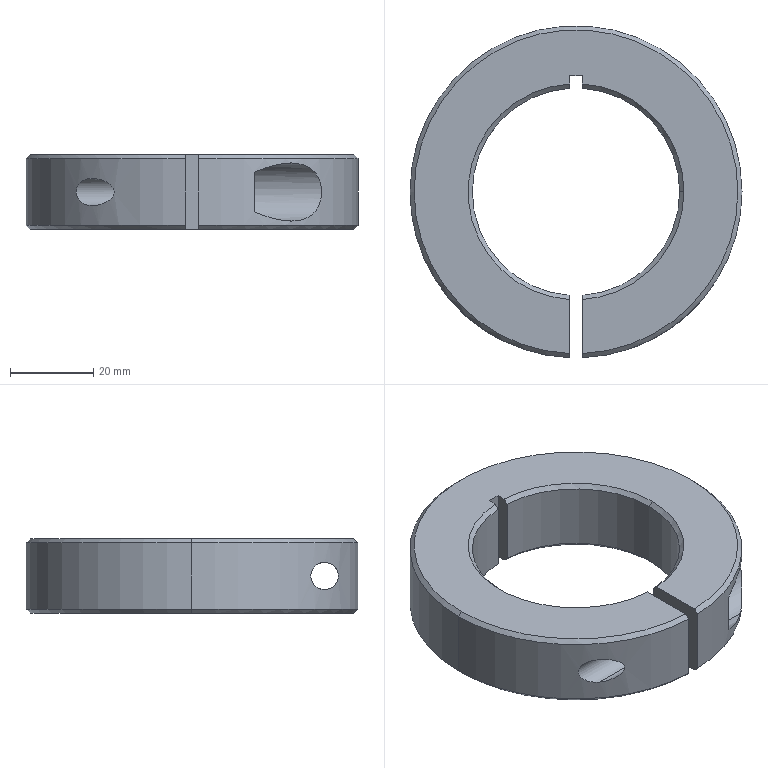Part | STEP file | SCSJ50_18b | 1 solid | 35 faces | box 80 x 79.972 x 18 mm | volume 50835 mm3 | cone 14 | cylinder 13 | plane 8 | commonest cylinder face diameters 14 x3 50 x3 80 x3 6.647 x2 9 x2